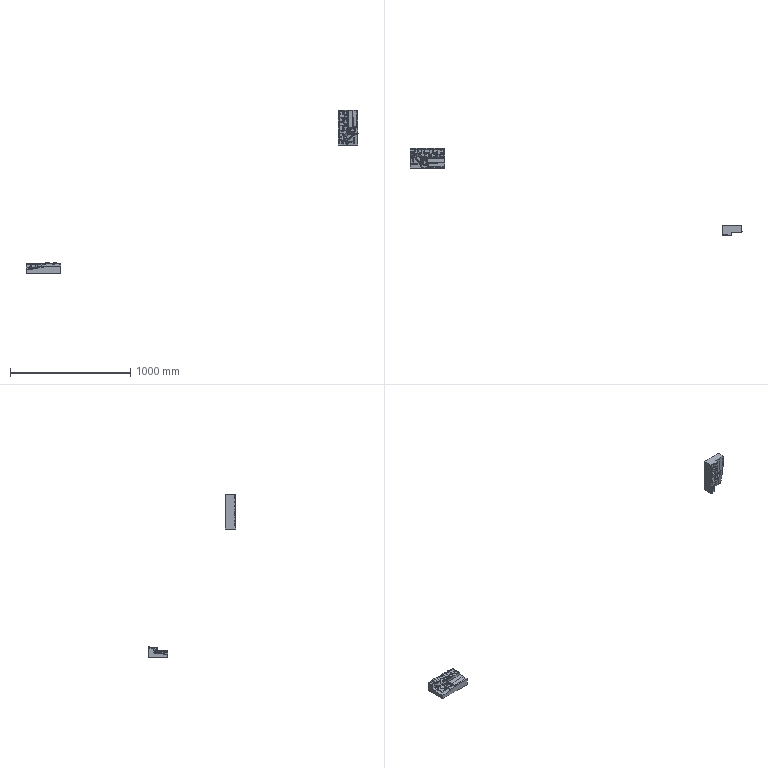NC program | NX | posted with a generic post | part box 2756 x 729.572 x 1353 mm
Lines 13207 to 14148 of 54396:
(CAVITY_MILL_1_COPY , TOOL : D12)
N26412 M6
N26414 G54
N26416 G17 G0 G90 X-61.78 Y-16.729 B0. C0. S3000 M3
N26418 G43 Z97. H0
N26420 Z88.089
N26422 G94 G1 Z87.889 F2500.
N26424 X-64.918 Y-10.686
N26426 G2 X-65.619 Y-7.821 R6.229
N26428 G1 X-65.626 Y-0.105
N26430 G2 X-64.958 Y2.719 R6.276
N26432 G1 X-61.892 Y8.823
N26434 Z88.089
N26436 G0 Z89.3
N26438 X-61.401 Y-17.106
N26440 Z87.534
N26442 G1 Z87.334
N26444 X-65.669 Y-11.752
N26446 G2 X-67.034 Y-8.198 R6.313
N26448 G1 X-67.043 Y-7.348
N26450 X-67.044 Y-0.546
N26452 X-67.036 Y0.304
N26454 G2 X-65.657 Y3.86 R6.363
N26456 G1 X-61.369 Y9.226
N26458 Z87.534
N26460 G0 Z88.745
N26462 X-21.599 Y-12.525
N26464 Z86.978
N26466 G1 Z86.778
N26468 X-28.34 Y-13.989
N26470 G2 X-29.835 Y-14.134 R6.429
N26472 G1 X-32.386 Y-14.139
N26474 X-60.453 Y-14.137
N26476 X-61.632 Y-14.135
N26478 G2 X-62.265 Y-14.102 R6.299
N26480 G1 X-69.575 Y-13.352
N26482 Z86.978
N26484 G0 Z88.745
N26486 X-20.318 Y-11.498
N26488 Z86.423
N26490 G1 Z86.223
N26492 X-26.744 Y-13.773
N26494 G2 X-28.813 Y-14.131 R6.245
N26496 G1 X-32.386 Y-14.139
N26498 X-60.453 Y-14.137
N26500 X-62.154 Y-14.135
N26502 G2 X-63.423 Y-14.028 R6.292
N26504 G1 X-73.529 Y-12.137
N26506 Z86.423
N26508 G0 Z97.
N26510 X-73.897 Y2.867
N26512 Z86.978
N26514 G1 Z86.778
N26516 X-73.91 Y-2.967
N26518 X-73.914 Y-4.897
N26520 G3 X-70.472 Y-9.44 R6.05
N26522 G2 X-69.563 Y-9.892 R16.839
N26524 X-66.657 Y-11.765 R17.425
N26526 G1 X-66.57 Y-11.833
N26528 G2 X-66.332 Y-12.019 R17.949
N26530 X-67.921 Y-7.835 R6.299
N26532 G1 X-67.919 Y-0.546
N26534 X-67.912 Y0.304
N26536 G2 X-66.243 Y4.227 R6.31
N26538 G1 X-61.593 Y9.25
N26540 Z86.978
N26542 G0 Z87.634
N26544 X-74.557 Y3.71
N26546 Z86.423
N26548 G1 Z86.223
N26550 Y-0.312
N26552 Y-7.552
N26554 G3 X-71.713 Y-9.641 R6.05
N26556 G2 X-69.34 Y-10.677 R17.426
N26558 X-66.7 Y-12.308 R18.024
N26560 X-68.557 Y-7.887 R6.292
N26562 G1 Y0.
N26564 G2 X-66.703 Y4.418 R6.295
N26566 G1 X-61.846 Y9.25
N26568 Z86.423
N26570 G0 Z97.
N26572 X-44.482 Y-49.697
N26574 Z84.757
N26576 G1 Z84.557
N26578 X-36.47 Y-46.781
N26580 G2 X-33.237 Y-46.149 R10.614
N26582 G1 X-32.386 Y-46.128
N26584 X-22.419 Y-46.233
N26586 X-16.419 Y-46.296
N26588 X-16.388 Y-43.296
N26590 Z84.757
N26592 G0 Z85.412
N26594 X-46.637 Y-51.248
N26596 Z84.201
N26598 G1 Z84.001
N26600 X-38.704 Y-46.644
N26602 G2 X-33.237 Y-45.076 R11.654
N26604 G1 X-32.386 Y-45.056
N26606 X-16.227 Y-45.086
N26608 X-15.376 Y-45.097
N26610 G2 X-14.979 Y-45.11 R11.508
N26612 G1 X-6.155 Y-45.55
N26614 Z84.201
N26616 G0 Z97.
N26618 X2.176 Y-65.002
N26620 Z82.454
N26622 G1 Z82.254
N26624 X-3.151 Y-73.288
N26626 G2 X-9.345 Y-78.601 R14.25
N26628 X-15.105 Y-79.966 R16.013
N26630 X-27.523 Y-80.461 R890.598
N26632 G1 X-27.676 Y-80.537
N26634 X-28.423 Y-80.799
N26636 X-34.085 Y-82.784
N26638 X-33.614 Y-85.487
N26640 Z82.454
N26642 G0 Z97.
N26644 X8.456 Y-82.827
N26646 Z64.573
N26648 G1 Z64.373
N26650 X1.996 Y-84.994
N26652 G2 X-0.067 Y-85.317 R6.238
N26654 G1 X-5.17
N26656 X-23.366 Y-85.394
N26658 X-29.366 Y-85.419
N26660 X-29.353 Y-88.419
N26662 Z64.573
N26664 G0 Z82.554
N26666 X9.055 Y-80.968
N26668 Z63.976
N26670 G1 Z63.776
N26672 X3.195 Y-84.444
N26674 G2 X-0.067 Y-85.317 R6.238
N26676 G1 X-5.17
N26678 X-46.403 Y-85.491
N26680 X-52.403 Y-85.516
N26682 X-52.39 Y-88.516
N26684 Z63.976
N26686 G0 Z82.554
N26688 X9.25 Y-78.495
N26690 Z63.38
N26692 G1 Z63.18
N26694 X4.499 Y-83.414
N26696 G2 X-0.067 Y-85.317 R6.237
N26698 G1 X-5.17
N26700 X-69.392 Y-85.588
N26702 X-75.392 Y-85.614
N26704 X-75.38 Y-88.613
N26706 Z63.38
N26708 G0 Z82.554
N26710 X9.25 Y-77.088
N26712 Z62.784
N26714 G1 Z62.584
N26716 X5.025 Y-82.793
N26718 G2 X-0.067 Y-85.317 R6.237
N26720 G1 X-5.17
N26722 X-71.51 Y-85.597
N26724 X-92.233 Y-85.683
N26726 X-98.233 Y-85.708
N26728 X-98.22 Y-88.708
N26730 Z62.784
N26732 G0 Z83.15
N26734 X9.25 Y-75.931
N26736 Z62.188
N26738 G1 Z61.988
N26740 X5.334 Y-82.334
N26742 G2 X-0.067 Y-85.317 R6.237
N26744 G1 X-5.17
N26746 X-67.257 Y-85.578
N26748 X-115.005 Y-85.776
N26750 X-121.005 Y-85.801
N26752 X-120.992 Y-88.801
N26754 Z62.188
N26756 G0 Z83.746
N26758 X9.25 Y-75.302
N26760 Z61.592
N26762 G1 Z61.392
N26764 X5.464 Y-82.112
N26766 G2 X-0.067 Y-85.318 R6.239
N26768 G1 X-5.17
N26770 X-67.257 Y-85.578
N26772 X-137.038 Y-85.868
N26774 X-143.038 Y-85.893
N26776 X-143.025 Y-88.893
N26778 Z61.592
N26780 G0 Z84.301
N26782 X9.25 Y-74.157
N26784 Z60.996
N26786 G1 Z60.796
N26788 X5.649 Y-81.766
N26790 G2 X-0.067 Y-85.342 R6.25
N26792 G1 X-10.273 Y-85.349
N26794 X-68.958 Y-85.588
N26796 X-148.096 Y-85.914
N26798 X-154.096 Y-85.939
N26800 X-154.089 Y-88.938
N26802 Z60.996
N26804 G0 Z85.412
N26806 X9.25 Y-71.875
N26808 Z60.4
N26810 G1 Z60.2
N26812 X5.889 Y-81.312
N26814 G2 X-0.067 Y-85.452 R6.232
N26816 G3 X-117.438 Y-85.79 R27313.051
N26818 G1 X-118.288 Y-85.795
N26820 X-157.412 Y-85.945
N26822 X-159.97 Y-85.949
N26824 X-165.97 Y-85.96
N26826 X-165.973 Y-88.96
N26828 Z60.4
N26830 G0 Z61.096
N26832 X-15.764 Y-92.815
N26834 Z59.804
N26836 G1 Z59.604
N26838 X-15.654 Y-91.659
N26840 X-9.654 Y-91.665
N26842 G2 X-1.342 Y-91.675 R24734.787
N26844 G3 X-0.921 Y-91.268 R6.05
N26846 G2 X0.288 Y-90.11 R15.727
N26848 G3 X0.763 Y-89.654 R6.05
N26850 G2 X2.921 Y-87.718 R16.428
N26852 G3 X5.144 Y-84.419 R6.05
N26854 G2 X5.621 Y-82.882 R18.634
N26856 G3 X5.899 Y-81.806 R6.05
N26858 G1 X5.999 Y-81.184
N26860 G2 X2.485 Y-85.151 R6.22
N26862 X-0.067 Y-85.677 R6.352
N26864 G3 X-154.01 Y-85.938 R24740.787
N26866 G1 X-161.471 Y-85.954
N26868 X-167.471 Y-85.967
N26870 X-167.533 Y-88.952
N26872 Z59.804
N26874 G0 Z60.5
N26876 X-28.81 Y-99.724
N26878 Z59.208
N26880 G1 Z59.008
N26882 X-25.562 Y-99.732
N26884 G2 X-10.79 Y-99.772 R26204.2
N26886 G1 X-11.54 Y-100.154
N26888 G2 X-25.019 Y-101.679 R357.943
N26890 G1 X-28.027 Y-101.962
N26892 Z59.208
N26894 G0 Z59.904
N26896 X-35.651 Y-93.708
N26898 Z59.208
N26900 G1 Z59.008
N26902 X-29.736 Y-93.722
N26904 G2 X-0.117 Y-93.806 R26210.2
N26906 G3 X0.311 Y-93.803 R14.049
N26908 G2 X1.794 Y-91.539 R14.616
N26910 G3 X2.238 Y-90.903 R6.05
N26912 G2 X3.301 Y-89.364 R15.564
N26914 G1 X3.404 Y-89.229
N26916 G2 X3.847 Y-88.658 R15.727
N26918 G3 X4.386 Y-87.878 R6.051
N26920 X5.095 Y-86.122 R6.05
N26922 G2 X5.148 Y-85.901 R18.075
N26924 G3 X5.268 Y-85.258 R6.05
N26926 G2 X5.844 Y-82.508 R18.634
N26928 G3 X6.051 Y-81.446 R6.051
N26930 G1 X6.064 Y-81.332
N26932 X6.073 Y-81.235
N26934 G2 X-0.067 Y-86.006 R6.249
N26936 G3 X-162.472 Y-85.955 R26218.
N26938 G1 X-168.472 Y-85.971
N26940 X-168.56 Y-88.937
N26942 Z59.208
N26944 G0 Z59.904
N26946 X1.758 Y-102.508
N26948 Z59.208
N26950 G1 Z59.008
N26952 X-1.237 Y-102.767
N26954 G3 X-6.066 Y-104.089 R13.915
N26956 G1 X-7.037 Y-104.594
N26958 X-9.731 Y-105.965
N26960 G2 X-25.118 Y-107.714 R363.943
N26962 X-31.541 Y-116.513 R14.06
N26964 G1 X-31.891 Y-116.724
N26966 X-32.966 Y-117.372
N26968 G3 X-33.483 Y-117.722 R6.05
N26970 X-34.592 Y-118.807 R6.05
N26972 G2 X-32.046 Y-116.973 R6.1
N26974 X-26.272 Y-115.649 R21.442
N26976 G3 X-8.117 Y-113.617 R371.743
N26978 G1 X-6.871 Y-113.262
N26980 X-3.469 Y-111.53
N26982 X-2.618 Y-111.088
N26984 G2 X4.02 Y-112.056 R6.115
N26986 G1 X9.104 Y-116.563
N26988 Z59.208
N26990 G0 Z60.5
N26992 X-51.654 Y-100.026
N26994 Z58.612
N26996 G1 Z58.412
N26998 X-48.428 Y-100.042
N27000 G2 X-44.367 Y-100.062 R16514.82
N27002 G1 X-34.644 Y-100.117
N27004 G3 X-35.492 Y-100.663 R64.118
N27006 G1 X-36.228 Y-100.782
N27008 X-47.917 Y-101.994
N27010 X-50.914 Y-102.305
N27012 Z58.612
N27014 G0 Z59.308
N27016 X-58.125 Y-93.995
N27018 Z58.612
N27020 G1 Z58.412
N27022 X-52.437 Y-94.022
N27024 G2 X-44.333 Y-94.062 R16520.821
N27026 G1 X-10.653 Y-94.253
N27028 X-2.883 Y-92.837
N27030 X-10.653 Y-94.253
N27032 X-14.264 Y-95.785
N27034 X-15.589 Y-96.389
N27036 X-15.95 Y-96.603
N27038 G2 X-21.97 Y-99.596 R45.827
N27040 G1 X-22.517 Y-99.82
N27042 X-23.753 Y-100.56
N27044 X-26.9 Y-102.598
N27046 G3 X-33.239 Y-106.375 R58.118
N27048 G1 X-35.435 Y-106.732
N27050 X-48.119 Y-108.047
N27052 G2 X-55.029 Y-116.919 R14.06
N27054 G1 X-56.264 Y-117.59
N27056 G3 X-56.964 Y-118.034 R6.051
N27058 G1 X-57.067 Y-118.107
N27060 G3 X-57.754 Y-118.675 R6.05
N27062 X-58.234 Y-119.191 R6.05
N27064 X-58.619 Y-119.709 R6.05
N27066 X-58.927 Y-120.228 R6.05
N27068 X-59.046 Y-120.466 R6.05
N27070 G2 X-55.321 Y-117.258 R6.111
N27072 G1 X-54.538 Y-117.018
N27074 X-50.806 Y-116.168
N27076 X-34.405 Y-114.467
N27078 X-31.716 Y-114.029
N27080 G3 X-29.026 Y-112.944 R6.587
N27082 G2 X-23.003 Y-109.367 R50.318
N27084 G1 X-19.629 Y-107.182
N27086 X-19.018 Y-106.816
N27088 G3 X-11.974 Y-103.313 R53.627
N27090 G1 X-11.124 Y-102.926
N27092 X-2.618 Y-99.318
N27094 X-1.768 Y-99.004
N27096 G2 X5.095 Y-101.564 R6.188
N27098 G1 X9.247 Y-107.898
N27100 Z58.612
N27102 G0 Z59.308
N27104 X9.25 Y-75.599
N27106 Z58.612
N27108 G1 Z58.412
N27110 X7.322
N27112 X6.123 Y-81.478
N27114 G2 X-0.067 Y-86.513 R6.293
N27116 G1 X-44.294 Y-86.262
N27118 G3 X-138.7 Y-86.042 R16528.621
N27120 G2 X-142.953 Y-85.901 R87.33
N27122 G1 X-163.322 Y-85.953
N27124 X-169.322 Y-85.968
N27126 X-169.428 Y-88.926
N27128 Z58.612
N27130 G0 Z83.746
N27132 X9.25 Y-76.056
N27134 Z58.016
N27136 G1 Z57.816
N27138 X7.154
N27140 X6.162 Y-81.973
N27142 G2 X1.529 Y-87.093 R6.404
N27144 X5.138 Y-89.813 R5.694
N27146 X5.962 Y-91.877 R7.348
N27148 G1 X7.319 Y-97.721
N27150 X9.25
N27152 Z58.016
N27154 G0 Z97.
N27156 X-74.455 Y-100.355
N27158 Z58.016
N27160 G1 Z57.816
N27162 X-71.25 Y-100.377
N27164 G2 X-58.564 Y-100.476 R11068.271
N27166 G1 X-59.375 Y-101.067
N27168 X-60.006 Y-101.187
N27170 X-70.777 Y-102.323
N27172 X-73.768 Y-102.638
N27174 Z58.016
N27176 G0 Z58.712
N27178 X-80.567 Y-94.313
N27180 Z58.016
N27182 G1 Z57.816
N27184 X-75.086 Y-94.351
N27186 G2 X-38.965 Y-94.656 R11074.271
N27188 G1 X-32.577 Y-93.181
N27190 X-38.965 Y-94.656
N27192 X-44.224 Y-97.759
N27194 G2 X-49.951 Y-101.411 R102.863
N27196 G3 X-53.73 Y-104.374 R17.847
N27198 G1 X-54.007 Y-104.578
N27200 X-56.93 Y-106.71
N27202 X-59.131 Y-107.128
N27204 X-71.082 Y-108.388
N27206 G2 X-78.315 Y-117.222 R14.06
N27208 G3 X-78.589 Y-117.369 R6.05
N27210 G2 X-79.402 Y-117.799 R14.616
N27212 G1 X-79.827 Y-118.009
N27214 G3 X-81.23 Y-118.966 R6.05
N27216 X-81.739 Y-119.482 R6.05
N27218 X-82.144 Y-119.999 R6.05
N27220 G1 X-82.201 Y-120.083
N27222 G2 X-79.262 Y-117.803 R6.053
N27224 X-73.831 Y-116.521 R24.233
N27226 G1 X-71.51 Y-116.249
N27228 X-58.752 Y-114.944
N27230 X-57.902 Y-114.834
N27232 X-53.864 Y-114.068
N27234 G2 X-53.649 Y-114.031 R-0.116
N27236 G1 X-53.163 Y-113.617
N27238 X-49.397 Y-110.87
N27240 X-48.51 Y-110.217
N27242 G2 X-45.995 Y-108.133 R10.047
N27244 G3 X-40.041 Y-104.348 R110.663
N27246 G1 X-34.139 Y-100.865
N27248 G3 X-21.33 Y-94.457 R266.162
N27250 G1 X-20.479 Y-94.098
N27252 X-4.319 Y-88.127
N27254 X-2.148 Y-87.288
N27256 G3 X-131.046 Y-86.31 R11082.071
N27258 G1 X-138.7 Y-86.291
N27260 X-140.401 Y-86.25
N27262 G3 X-143.804 Y-85.906 R269.67
N27264 G1 X-166.766 Y-85.958
N27266 X-172.766 Y-85.972
N27268 X-173.004 Y-88.742
N27270 Z58.016
N27272 G0 Z58.712
N27274 X-97.072 Y-100.739
N27276 Z57.42
N27278 G1 Z57.22
N27280 X-93.892 Y-100.771
N27282 G2 X-83.193 Y-100.889 R6665.304
N27284 X-83.992 Y-101.658 R125.953
N27286 G1 X-85.686 Y-101.822
N27288 X-93.474 Y-102.648
N27290 X-96.461 Y-102.964
N27292 Z57.42
N27294 G0 Z58.116
N27296 X-102.782 Y-94.684
N27298 Z57.42
N27300 G1 Z57.22
N27302 X-97.517 Y-94.735
N27304 G2 X-67.8 Y-95.089 R6671.304
N27306 G1 X-62.006 Y-93.396
N27308 X-67.8 Y-95.089
N27310 G3 X-71.268 Y-97.878 R20.699
N27312 G2 X-74.41 Y-100.641 R32.752
N27314 G1 X-74.884 Y-101.007
N27316 X-75.296 Y-101.44
N27318 G2 X-81.163 Y-107.233 R131.953
N27320 G1 X-82.996 Y-107.59
N27322 X-85.054 Y-107.789
N27324 X-93.885 Y-108.725
N27326 G2 X-101.022 Y-117.304 R14.06
N27328 G3 X-101.293 Y-117.45 R6.05
N27330 G2 X-102.648 Y-118.135 R14.616
N27332 X-102.117 Y-117.981 R6.089
N27334 G1 X-98.126 Y-117.018
N27336 X-84.268 Y-115.549
N27338 X-81.874 Y-115.318
N27340 X-78.314 Y-114.625
N27342 X-77.519 Y-114.467
N27344 G3 X-69.645 Y-106.816 R139.753
N27346 X-65.754 Y-103.395 R40.552
N27348 G2 X-62.166 Y-100.865 R12.899
N27350 X-46.845 Y-90.779 R239.385
N27352 G1 X-46.623 Y-90.663
N27354 X-39.846 Y-87.741
N27356 G3 X-139.551 Y-86.66 R6679.104
N27358 G2 X-143.126 Y-86.139 R19.306
N27360 G3 X-145.062 Y-85.91 R8.098
N27362 G1 X-162.515 Y-85.962
N27364 G2 X-172.721 Y-85.8 R93.182
N27366 X-188.488 Y-82.3 R56.907
N27368 G1 X-194.102 Y-80.182
N27370 X-195.323 Y-82.564
N27372 Z57.42
N27374 G0 Z58.116
N27376 X-119.348 Y-101.204
N27378 Z56.824
N27380 G1 Z56.624
N27382 X-116.198 Y-101.248
N27384 G2 X-108.784 Y-101.362 R3537.579
N27386 X-109.321 Y-102.27 R65.524
N27388 G1 X-115.856 Y-102.961
N27390 X-118.841 Y-103.276
N27392 Z56.824
N27394 G0 Z57.52
N27396 X-124.508 Y-95.136
N27398 Z56.824
N27400 G1 Z56.624
N27402 X-119.565 Y-95.202
N27404 G2 X-96.909 Y-95.574 R3543.579
N27406 G1 X-101.094 Y-100.202
N27408 X-101.968 Y-101.413
N27410 X-102.221 Y-101.893
N27412 G2 X-105.738 Y-107.836 R71.524
N27414 G1 X-106.687 Y-108.026
N27416 X-116.368 Y-109.048
N27418 G2 X-123.154 Y-117.251 R14.06
N27420 G3 X-123.409 Y-117.396 R6.05
N27422 G2 X-125.341 Y-118.367 R14.616
N27424 G1 X-126.185 Y-118.715
N27426 G3 X-128.195 Y-120.071 R6.05
N27428 G2 X-126.269 Y-118.769 R6.004
N27430 X-121.143 Y-117.395 R19.238
N27432 G1 X-118.102 Y-117.018
N27434 X-105.53 Y-115.748
N27436 X-101.501 Y-114.945
N27438 X-101.491 Y-114.779
N27440 X-101.129 Y-114.89
N27442 G3 X-95.324 Y-105.536 R79.324
N27444 G1 X-95.021 Y-105.116
N27446 X-91.072 Y-100.752
N27448 X-89.022 Y-98.315
N27450 X-88.52 Y-97.832
N27452 G3 X-83.665 Y-93.214 R38.829
N27454 G2 X-81.451 Y-90.833 R6.958
N27456 G1 X-77.493 Y-88.207
N27458 G3 X-139.416 Y-87.194 R3551.379
N27460 G2 X-141.448 Y-86.957 R9.468
N27462 X-144.106 Y-86.167 R21.42
N27464 G3 X-145.54 Y-85.913 R4.106
N27466 G1 X-159.963 Y-85.957
N27468 X-160.814 Y-85.977
N27470 X-161.664 Y-86.011
N27472 G2 X-171.87 Y-85.94 R103.168
N27474 X-187.667 Y-82.774 R57.83
N27476 G1 X-193.328 Y-80.787
N27478 X-194.488 Y-83.204
N27480 Z56.824
N27482 G0 Z57.52
N27484 X-140.634 Y-95.834
N27486 Z56.228
N27488 G1 Z56.028
N27490 X-136.324 Y-95.957
N27492 X-127.81 Y-96.202
N27494 X-128.693 Y-97.748
N27496 G3 X-130.305 Y-102.136 R14.089
N27498 G2 X-131.686 Y-108.71 R153.814
N27500 G1 X-133.819 Y-108.958
N27502 G2 X-139.098 Y-116.615 R14.616
N27504 G3 X-139.367 Y-116.83 R6.05
N27506 G2 X-140.823 Y-117.918 R15.564
N27508 X-138.708 Y-117.317 R7.283
N27510 G1 X-138.7 Y-117.379
N27512 X-128.296 Y-116.168
N27514 X-125.373 Y-115.604
N27516 G3 X-122.638 Y-103.573 R161.614
N27518 G2 X-121.919 Y-101.614 R6.289
N27520 G1 X-119.989 Y-98.234
N27522 X-119.66 Y-97.464
N27524 G2 X-117.308 Y-92.363 R13.177
N27526 X-115.659 Y-88.747 R8.523
N27528 G1 X-139.551 Y-88.062
N27530 X-140.401 Y-87.973
N27532 G2 X-144.654 Y-86.343 R13.748
N27534 G1 X-144.914 Y-86.2
N27536 G3 X-145.505 Y-86.009 R1.232
N27538 X-157.412 Y-85.956 R460.851
N27540 G1 X-158.262 Y-85.983
N27542 X-164.216 Y-86.227
N27544 G2 X-173.571 Y-85.954 R85.991
N27546 X-183.753 Y-84.164 R57.271
N27548 G1 X-189.544 Y-82.596
N27550 X-190.502 Y-85.122
N27552 Z56.228
N27554 G0 Z56.924
N27556 X-148.804 Y-109.141
N27558 Z55.632
N27560 G1 Z55.432
N27562 X-145.804 Y-109.079
N27564 X-145.929 Y-103.08
N27566 X-146.282 Y-86.175
N27568 G3 X-153.803 Y-86.037 R549.543
N27570 X-161.276 Y-86.285 R83.619
N27572 G2 X-167.921 Y-86.449 R62.384
N27574 G1 X-173.918 Y-86.277
N27576 X-174.168 Y-89.102
N27578 Z55.632
N27580 G0 Z56.328
N27582 X-150.073 Y-109.246
N27584 Z55.036
N27586 G1 Z54.836
N27588 X-147.073 Y-109.194
N27590 X-147.178 Y-103.195
N27592 X-147.458 Y-87.262
N27594 X-147.478 Y-86.432
N27596 X-154.01 Y-86.224
N27598 X-154.86 Y-86.205
N27600 G3 X-160.814 Y-86.523 R66.368
N27602 G2 X-167.618 Y-86.74 R52.243
N27604 G1 X-168.468 Y-86.709
N27606 G2 X-171.673 Y-86.545 R104.994
N27608 G1 X-177.66 Y-86.146
N27610 X-178.081 Y-88.91
N27612 Z55.036
N27614 G0 Z55.732
N27616 X-150.824 Y-109.807
N27618 Z54.44
N27620 G1 Z54.24
N27622 X-147.825 Y-109.757
N27624 X-147.926 Y-103.758
N27626 X-148.212 Y-86.822
N27628 X-154.86 Y-86.516
N27630 X-155.711 Y-86.517
N27632 G3 X-162.515 Y-87.014 R110.545
N27634 G2 X-169.465 Y-87.016 R51.443
N27636 G1 X-169.721 Y-90.005
N27638 Z54.44
N27640 G0 Z56.924
N27642 X-133.429 Y-173.75
N27644 Z53.844
N27646 G1 Z53.644
N27648 X-143.633 Y-170.399
N27650 G2 X-147.912 Y-164.941 R6.246
N27652 G1 X-147.936 Y-164.627
N27654 X-149.126 Y-87.355
N27656 X-154.86 Y-86.957
N27658 G3 X-160.145 Y-87.262 R42.844
N27660 G2 X-169.319 Y-87.44 R43.731
N27662 X-173.688 Y-87.132 R83.341
N27664 G1 X-179.66 Y-86.553
N27666 X-180.181 Y-89.287
N27668 Z53.844
N27670 G0 Z54.54
N27672 X-153.927 Y-109.239
N27674 Z53.248
N27676 G1 Z53.048
N27678 X-150.927 Y-109.226
N27680 X-150.954 Y-103.226
N27682 X-151.017 Y-88.963
N27684 X-150.953 Y-88.093
N27686 G3 X-159.762 Y-87.855 R27.454
N27688 G2 X-167.635 Y-88.105 R38.477
N27690 G1 X-171.574 Y-87.826
N27692 G2 X-173.876 Y-87.627 R76.183
N27694 G1 X-179.845 Y-87.021
N27696 X-180.339 Y-89.741
N27698 Z53.248
N27700 G0 Z53.944
N27702 X-158.257 Y-101.682
N27704 Z52.652
N27706 G1 Z52.452
N27708 X-155.804 Y-100.265
N27710 X-157.303 Y-97.667
N27712 G2 X-158.704 Y-94.064 R12.733
N27714 G1 X-158.762 Y-93.214
N27716 X-158.739 Y-88.963
N27718 Y-88.697
N27720 G2 X-170.169 Y-88.604 R44.8
N27722 X-179.525 Y-87.457 R98.024
N27724 X-180.143 Y-87.331 R54.169
N27726 G1 X-186.015 Y-86.099
N27728 X-186.847 Y-88.635
N27730 Z52.652
N27732 G0 Z53.348
N27734 X-157.411 Y-117.241
N27736 Z52.056
N27738 G1 Z51.856
N27740 X-154.411 Y-117.19
N27742 X-154.512 Y-111.191
N27744 X-154.585 Y-106.89
N27746 G3 X-157.688 Y-99.516 R10.744
N27748 X-161.002 Y-96.977 R15.271
N27750 G2 X-161.403 Y-96.744 R23.046
N27752 G1 X-166.559 Y-93.675
N27754 X-167.896 Y-95.54
N27756 Z52.056
N27758 G0 Z97.
N27760 X-161.905 Y-100.211
N27762 Z52.056
N27764 G1 Z51.856
N27766 X-160.579 Y-98.8
N27768 X-164.618 Y-94.363
N27770 G2 X-166.481 Y-90.157 R7.276
N27772 G1 X-176.123 Y-88.786
N27774 G2 X-180.764 Y-87.925 R54.14
N27776 G1 X-186.61 Y-86.575
N27778 X-187.493 Y-89.093
N27780 Z52.056
N27782 G0 Z52.752
N27784 X-167.774 Y-99.603
N27786 Z51.46
N27788 G1 Z51.26
N27790 X-172.41 Y-93.722
N27792 G2 X-173.835 Y-90.336 R6.902
N27794 X-189.034 Y-86.076 R66.474
N27796 G1 X-194.578 Y-83.782
N27798 X-195.907 Y-86.089
N27800 Z51.46
N27802 G0 Z52.156
N27804 X-176.281 Y-101.203
N27806 Z50.864
N27808 G1 Z50.664
N27810 X-179.975 Y-95.193
N27812 G2 X-180.797 Y-93.214 R6.841
N27814 X-180.92 Y-90.243 R15.454
N27816 X-194.857 Y-84.1 R71.543
N27818 G1 X-200.058 Y-81.109
N27820 X-201.568 Y-82.812
N27822 Z50.864
N27824 G0 Z51.56
N27826 X-187.744 Y-106.272
N27828 Z50.268
N27830 G1 Z50.068
N27832 X-187.72 Y-97.721
N27834 X-187.697 Y-89.312
N27836 G2 X-196.535 Y-84.151 R99.795
N27838 X-201.074 Y-79.856 R41.784
N27840 X-205.612 Y-76.537 R58.406
N27842 G1 X-207.947 Y-74.653
N27844 X-209.825 Y-77.001
N27846 Z50.268
N27848 G0 Z50.964
N27850 X-197.159 Y-97.123
N27852 Z49.671
N27854 G1 Z49.471
N27856 X-194.147 Y-97.133
N27858 X-194.163 Y-94.133
N27860 X-194.2 Y-87.535
N27862 X-197.386 Y-85.041
N27864 G2 X-201.44 Y-80.296 R50.694
N27866 X-205.891 Y-76.949 R53.52
N27868 G1 X-206.438 Y-76.486
N27870 X-208.402 Y-78.754
N27872 Z49.671
N27874 G0 Z50.368
N27876 X-203.326 Y-95.424
N27878 Z49.075
N27880 G1 Z48.875
N27882 X-200.326 Y-95.427
N27884 X-200.32 Y-89.427
N27886 X-200.315 Y-84.712
N27888 X-200.369 Y-83.862
N27890 X-200.384 Y-83.763
N27892 X-201.638 Y-81.24
N27894 X-201.913 Y-80.801
N27896 G2 X-206.741 Y-76.97 R58.051
N27898 G1 X-206.947 Y-76.791
N27900 X-209.004 Y-78.977
N27902 Z49.075
N27904 G0 Z49.771
N27906 X-205.527 Y-94.418
N27908 Z48.479
N27910 G1 Z48.279
N27912 X-202.527 Y-94.419
N27914 X-202.526 Y-88.419
N27916 Y-81.493
N27918 X-202.52 Y-81.387
N27920 X-202.607 Y-81.326
N27922 G2 X-207.78 Y-76.933 R94.276
N27924 G1 X-209.889 Y-79.07
N27926 Z48.479
N27928 G0 Z49.175
N27930 X-206.713 Y-93.652
N27932 Z47.883
N27934 G1 Z47.683
N27936 X-203.713 Y-93.653
N27938 X-203.711 Y-87.653
N27940 X-203.709 Y-81.742
N27942 X-205.04 Y-80.549
N27944 X-207.951 Y-77.839
N27946 X-210.146 Y-75.795
N27948 X-212.191 Y-77.99
N27950 Z47.883
N27952 G0 Z48.579
N27954 X-208.002 Y-93.949
N27956 Z47.287
N27958 G1 Z47.087
N27960 X-205.002
N27962 Y-87.949
N27964 Y-83.012
N27966 X-204.993 Y-82.377
N27968 G3 X-211.088 Y-76.024 R124.193
N27970 G1 X-213.19 Y-78.164
N27972 Z47.287
N27974 G0 Z47.983
N27976 X-211.279 Y-92.608
N27978 Z46.691
N27980 G1 Z46.491
N27982 X-208.279
N27984 Y-86.608
N27986 Y-81.147
N27988 G3 X-213.119 Y-75.36 R34.219
N27990 G1 X-213.989 Y-74.51
N27992 X-214.609 Y-73.931
N27994 X-218.996 Y-69.836
N27996 X-221.043 Y-72.029
N27998 Z46.691
N28000 G0 Z47.387
N28002 X-215.121 Y-90.203
N28004 Z46.095
N28006 G1 Z45.895
N28008 X-212.121 Y-90.202
N28010 X-212.123 Y-84.202
N28012 X-212.124 Y-78.742
N28014 G3 X-214.716 Y-75.346 R21.007
N28016 G1 X-216.299 Y-73.66
N28018 X-217.941 Y-72.049
N28020 X-220.082 Y-69.947
N28022 X-222.183 Y-72.088
N28024 Z46.095
N28026 G0 Z46.791
N28028 X-218.967 Y-87.742
N28030 Z45.499
N28032 G1 Z45.299
N28034 X-215.967
N28036 X-215.968 Y-81.742
N28038 Y-76.395
N28040 G3 X-219.499 Y-71.947 R29.448
N28042 X-223.182 Y-68.189 R35.96
N28044 G1 X-225.18 Y-70.426
N28046 Z45.499
N28048 G0 Z46.195
N28050 X-222.813 Y-85.315
N28052 Z44.903
N28054 G1 Z44.703
N28056 X-219.813
N28058 Y-79.315
N28060 Y-74.088
N28062 G3 X-231.662 Y-63.389 R28.524
N28064 G1 X-234.572 Y-61.98
N28066 X-237.272 Y-60.673
N28068 X-238.579 Y-63.373
N28070 Z44.903
N28072 G0 Z97.
N28074 X-15.259 Y-123.158
N28076 Z59.804
N28078 G1 Z59.604
N28080 X-10.746 Y-118.196
N28082 G2 X-8.68 Y-116.724 R5.979
N28084 X-5.17 Y-115.718 R14.498
N28086 X-0.917 Y-115.083 R18.515
N28088 G1 X-0.332 Y-115.045
N28090 G2 X2.499 Y-115.542 R6.074
N28092 G1 X8.674 Y-118.246
N28094 Z59.804
N28096 G0 Z97.
N28098 X-23.8 Y-83.63
N28100 Z82.454
N28102 G1 Z82.254
N28104 X-29.153 Y-80.91
N28106 X-29.835 Y-80.564
N28108 X-30.6 Y-80.683
N28110 G2 X-31.865 Y-81.682 R6.53
N28112 G1 X-38.109 Y-85.468
N28114 Z82.454
N28116 G0 Z97.
N28118 X-41.302 Y-75.599
N28120 Z84.757
N28122 G1 Z84.557
N28124 X-43.131 Y-67.276
N28126 G2 X-43.33 Y-66.009 R10.604
N28128 G1 X-43.402 Y-65.158
N28130 X-43.466 Y-56.657
N28132 X-43.443 Y-56.267
N28134 G2 X-43.242 Y-54.641 R10.614
N28136 G1 X-41.544 Y-46.287
N28138 Z84.757
N28140 G0 Z85.412
N28142 X-39.429 Y-78.107
N28144 Z84.201
N28146 G1 Z84.001
N28148 X-43.299 Y-70.095
N28150 G2 X-44.462 Y-65.158 R11.695
N28152 G1 X-44.514 Y-57.507
N28154 X-44.508 Y-56.657
N28156 G2 X-43.42 Y-51.808 R11.654
N28158 G1 X-39.593 Y-43.581
N28160 Z84.201
N28162 G0 Z84.857
N28164 X-20.416 Y-36.562
N28166 Z83.646
N28168 G1 Z83.446
N28170 X-24.39 Y-36.561
N28172 X-32.32 Y-36.56
N28174 G3 X-32.528 Y-36.558 R20.968
N28176 G1 X-36.314 Y-36.539
N28178 Z83.646
N28180 G0 Z85.412
N28182 X-28.282 Y-80.357
N28184 Z83.646
N28186 G1 Z83.446
N28188 X-37.67 Y-76.432
N28190 G2 X-43.126 Y-71.96 R12.311
N28192 X-45.123 Y-65.863 R12.816
N28194 G1 X-45.168 Y-65.158
N28196 X-45.23 Y-56.657
N28198 X-45.144 Y-55.583
N28200 G2 X-35.788 Y-44.721 R12.018
N28202 G1 X-34.938 Y-44.561
N28204 G2 X-32.386 Y-44.36 R13.168
N28206 G1 X-15.728 Y-44.363
N28208 G2 X-9.371 Y-46.007 R13.116
N28210 G1 X-1.625 Y-50.301
N28212 Z83.646
N28214 G0 Z85.412
N28216 X-54.056 Y-53.176
N28218 Z83.05
N28220 G1 Z82.85
N28222 X-54.022 Y-57.062
N28224 X-53.954 Y-64.833
N28226 G3 X-51.502 Y-66.562 R6.05
N28228 G2 X-46.484 Y-69.601 R16.282
N28230 X-44.239 Y-72.041 R16.272
N28232 X-46.151 Y-65.158 R13.768
N28234 G1 X-46.225 Y-56.657
N28236 X-46.204 Y-56.047
N28238 G2 X-44.274 Y-49.638 R13.143
N28240 G1 X-41.138 Y-44.522
N28242 X-42.266 Y-43.209
N28244 Z83.05
N28246 G0 Z97.
N28248 X-74.867 Y-44.324
N28250 Z84.201
N28252 G1 Z84.001
N28254 X-71.237 Y-52.277
N28256 G2 X-70.227 Y-56.657 R11.238
N28258 G1 X-70.214 Y-57.507
N28260 X-70.201 Y-65.158
N28262 X-70.225 Y-65.761
N28264 G2 X-71.15 Y-69.763 R11.109
N28266 G1 X-74.64 Y-77.73
N28268 Z84.201
N28270 G0 Z84.857
N28272 X-63.502 Y-68.287
N28274 Z83.646
N28276 G1 Z83.446
N28278 X-63.388 Y-63.533
N28280 G3 X-63.413 Y-58.444 R88.311
N28282 X-65.713 Y-55.866 R6.05
N28284 G2 X-67.719 Y-54.399 R15.727
N28286 G1 X-67.828 Y-54.307
N28288 G2 X-71.1 Y-50.677 R16.353